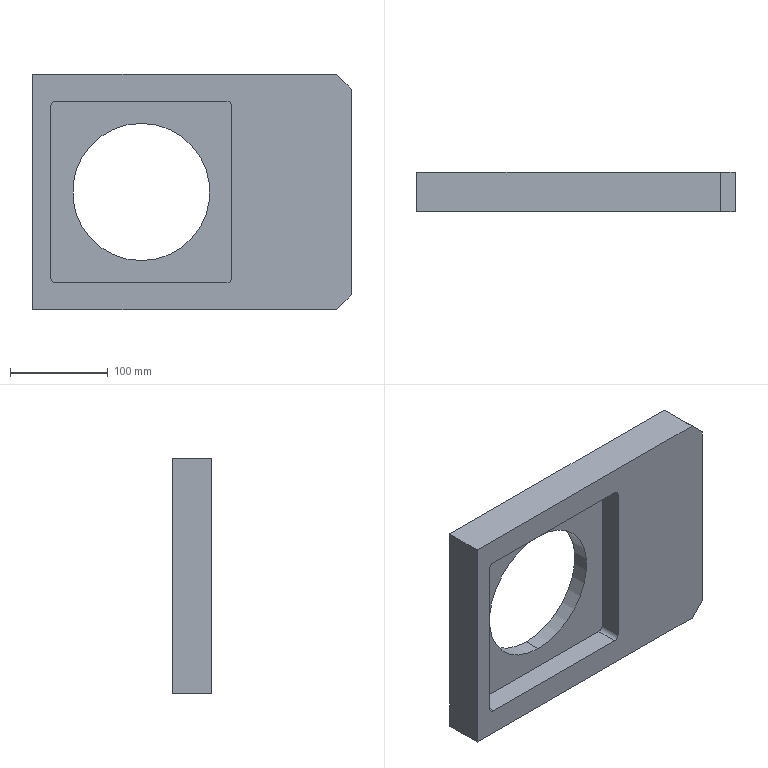Part | SolidWorks | features Cut 2, Chamfer 1, Extrusion 1, Fillet 1 | 1 solid | 19 faces | box 325 x 40 x 240 mm | volume 2062624 mm3 | plane 13 | cylinder 6 | commonest cylinder face diameters 10 x4 140 x2
STEP:
#1=CARTESIAN_POINT('',(-51.794,40.,70.));
#2=VERTEX_POINT('',#1);
#3=CARTESIAN_POINT('',(-51.794,40.,-70.));
#4=VERTEX_POINT('',#3);
#5=CARTESIAN_POINT('',(-51.794,40.,0.));
#6=DIRECTION('',(0.,-1.,0.));
#7=DIRECTION('',(0.,0.,-1.));
#8=AXIS2_PLACEMENT_3D('',#5,#6,#7);
#9=CIRCLE('',#8,70.);
#10=EDGE_CURVE('',#2,#4,#9,.T.);
#11=ORIENTED_EDGE('',*,*,#10,.F.);
#12=CARTESIAN_POINT('',(-51.794,23.,70.));
#13=VERTEX_POINT('',#12);
#14=CARTESIAN_POINT('',(-51.794,40.,70.));
#15=DIRECTION('',(0.,-1.,0.));
#16=VECTOR('',#15,1000.);
#17=LINE('',#14,#16);
#18=EDGE_CURVE('',#2,#13,#17,.T.);
#19=ORIENTED_EDGE('',*,*,#18,.T.);
#20=CARTESIAN_POINT('',(-51.794,23.,-70.));
#21=VERTEX_POINT('',#20);
#22=CARTESIAN_POINT('',(-51.794,23.,0.));
#23=DIRECTION('',(0.,-1.,0.));
#24=DIRECTION('',(0.,0.,-1.));
#25=AXIS2_PLACEMENT_3D('',#22,#23,#24);
#26=CIRCLE('',#25,70.);
#27=EDGE_CURVE('',#13,#21,#26,.T.);
#28=ORIENTED_EDGE('',*,*,#27,.T.);
#29=CARTESIAN_POINT('',(-51.794,40.,-70.));
#30=DIRECTION('',(0.,-1.,0.));
#31=VECTOR('',#30,1000.);
#32=LINE('',#29,#31);
#33=EDGE_CURVE('',#4,#21,#32,.T.);
#34=ORIENTED_EDGE('',*,*,#33,.F.);
#35=EDGE_LOOP('',(#11,#19,#28,#34));
#36=FACE_OUTER_BOUND('',#35,.T.);
#37=CARTESIAN_POINT('',(-51.794,40.,0.));
#38=DIRECTION('',(0.,-1.,0.));
#39=DIRECTION('',(0.,0.,-1.));
#40=AXIS2_PLACEMENT_3D('',#37,#38,#39);
#41=CYLINDRICAL_SURFACE('',#40,70.);
#42=ADVANCED_FACE('',(#36),#41,.F.);
#43=CARTESIAN_POINT('',(162.5,0.,105.));
#44=VERTEX_POINT('',#43);
#45=CARTESIAN_POINT('',(162.5,0.,-105.));
#46=VERTEX_POINT('',#45);
#47=CARTESIAN_POINT('',(162.5,0.,120.));
#48=DIRECTION('',(0.,0.,-1.));
#49=VECTOR('',#48,1000.);
#50=LINE('',#47,#49);
#51=EDGE_CURVE('',#44,#46,#50,.T.);
#52=ORIENTED_EDGE('',*,*,#51,.T.);
#53=CARTESIAN_POINT('',(162.5,40.,-105.));
#54=VERTEX_POINT('',#53);
#55=CARTESIAN_POINT('',(162.5,40.,-105.));
#56=DIRECTION('',(0.,1.,0.));
#57=VECTOR('',#56,1000.);
#58=LINE('',#55,#57);
#59=EDGE_CURVE('',#46,#54,#58,.T.);
#60=ORIENTED_EDGE('',*,*,#59,.T.);
#61=CARTESIAN_POINT('',(162.5,40.,105.));
#62=VERTEX_POINT('',#61);
#63=CARTESIAN_POINT('',(162.5,40.,120.));
#64=DIRECTION('',(0.,0.,-1.));
#65=VECTOR('',#64,1000.);
#66=LINE('',#63,#65);
#67=EDGE_CURVE('',#62,#54,#66,.T.);
#68=ORIENTED_EDGE('',*,*,#67,.F.);
#69=CARTESIAN_POINT('',(162.5,40.,105.));
#70=DIRECTION('',(0.,-1.,0.));
#71=VECTOR('',#70,1000.);
#72=LINE('',#69,#71);
#73=EDGE_CURVE('',#62,#44,#72,.T.);
#74=ORIENTED_EDGE('',*,*,#73,.T.);
#75=EDGE_LOOP('',(#52,#60,#68,#74));
#76=FACE_OUTER_BOUND('',#75,.T.);
#77=CARTESIAN_POINT('',(162.5,40.,120.));
#78=DIRECTION('',(-1.,0.,0.));
#79=DIRECTION('',(0.,0.,1.));
#80=AXIS2_PLACEMENT_3D('',#77,#78,#79);
#81=PLANE('',#80);
#82=ADVANCED_FACE('',(#76),#81,.F.);
#83=CARTESIAN_POINT('',(147.5,40.,-120.));
#84=VERTEX_POINT('',#83);
#85=CARTESIAN_POINT('',(-162.5,40.,-120.));
#86=VERTEX_POINT('',#85);
#87=CARTESIAN_POINT('',(-162.5,40.,-120.));
#88=DIRECTION('',(-1.,0.,0.));
#89=VECTOR('',#88,1000.);
#90=LINE('',#87,#89);
#91=EDGE_CURVE('',#84,#86,#90,.T.);
#92=ORIENTED_EDGE('',*,*,#91,.F.);
#93=CARTESIAN_POINT('',(147.5,0.,-120.));
#94=VERTEX_POINT('',#93);
#95=CARTESIAN_POINT('',(147.5,40.,-120.));
#96=DIRECTION('',(0.,-1.,0.));
#97=VECTOR('',#96,1000.);
#98=LINE('',#95,#97);
#99=EDGE_CURVE('',#84,#94,#98,.T.);
#100=ORIENTED_EDGE('',*,*,#99,.T.);
#101=CARTESIAN_POINT('',(-162.5,0.,-120.));
#102=VERTEX_POINT('',#101);
#103=CARTESIAN_POINT('',(-162.5,0.,-120.));
#104=DIRECTION('',(-1.,0.,0.));
#105=VECTOR('',#104,1000.);
#106=LINE('',#103,#105);
#107=EDGE_CURVE('',#94,#102,#106,.T.);
#108=ORIENTED_EDGE('',*,*,#107,.T.);
#109=CARTESIAN_POINT('',(-162.5,40.,-120.));
#110=DIRECTION('',(0.,-1.,0.));
#111=VECTOR('',#110,1000.);
#112=LINE('',#109,#111);
#113=EDGE_CURVE('',#86,#102,#112,.T.);
#114=ORIENTED_EDGE('',*,*,#113,.F.);
#115=EDGE_LOOP('',(#92,#100,#108,#114));
#116=FACE_OUTER_BOUND('',#115,.T.);
#117=CARTESIAN_POINT('',(-162.5,40.,-120.));
#118=DIRECTION('',(0.,0.,1.));
#119=DIRECTION('',(1.,0.,0.));
#120=AXIS2_PLACEMENT_3D('',#117,#118,#119);
#121=PLANE('',#120);
#122=ADVANCED_FACE('',(#116),#121,.F.);
#123=CARTESIAN_POINT('',(-162.5,0.,120.));
#124=VERTEX_POINT('',#123);
#125=CARTESIAN_POINT('',(-162.5,0.,120.));
#126=DIRECTION('',(0.,0.,1.));
#127=VECTOR('',#126,1000.);
#128=LINE('',#125,#127);
#129=EDGE_CURVE('',#102,#124,#128,.T.);
#130=ORIENTED_EDGE('',*,*,#129,.T.);
#131=CARTESIAN_POINT('',(-162.5,40.,120.));
#132=VERTEX_POINT('',#131);
#133=CARTESIAN_POINT('',(-162.5,40.,120.));
#134=DIRECTION('',(0.,-1.,0.));
#135=VECTOR('',#134,1000.);
#136=LINE('',#133,#135);
#137=EDGE_CURVE('',#132,#124,#136,.T.);
#138=ORIENTED_EDGE('',*,*,#137,.F.);
#139=CARTESIAN_POINT('',(-162.5,40.,120.));
#140=DIRECTION('',(0.,0.,1.));
#141=VECTOR('',#140,1000.);
#142=LINE('',#139,#141);
#143=EDGE_CURVE('',#86,#132,#142,.T.);
#144=ORIENTED_EDGE('',*,*,#143,.F.);
#145=ORIENTED_EDGE('',*,*,#113,.T.);
#146=EDGE_LOOP('',(#130,#138,#144,#145));
#147=FACE_OUTER_BOUND('',#146,.T.);
#148=CARTESIAN_POINT('',(-162.5,40.,120.));
#149=DIRECTION('',(1.,0.,0.));
#150=DIRECTION('',(0.,0.,-1.));
#151=AXIS2_PLACEMENT_3D('',#148,#149,#150);
#152=PLANE('',#151);
#153=ADVANCED_FACE('',(#147),#152,.F.);
#154=CARTESIAN_POINT('',(147.5,0.,120.));
#155=VERTEX_POINT('',#154);
#156=CARTESIAN_POINT('',(-162.5,0.,120.));
#157=DIRECTION('',(1.,0.,0.));
#158=VECTOR('',#157,1000.);
#159=LINE('',#156,#158);
#160=EDGE_CURVE('',#124,#155,#159,.T.);
#161=ORIENTED_EDGE('',*,*,#160,.T.);
#162=CARTESIAN_POINT('',(147.5,40.,120.));
#163=VERTEX_POINT('',#162);
#164=CARTESIAN_POINT('',(147.5,40.,120.));
#165=DIRECTION('',(0.,1.,0.));
#166=VECTOR('',#165,1000.);
#167=LINE('',#164,#166);
#168=EDGE_CURVE('',#155,#163,#167,.T.);
#169=ORIENTED_EDGE('',*,*,#168,.T.);
#170=CARTESIAN_POINT('',(-162.5,40.,120.));
#171=DIRECTION('',(1.,0.,0.));
#172=VECTOR('',#171,1000.);
#173=LINE('',#170,#172);
#174=EDGE_CURVE('',#132,#163,#173,.T.);
#175=ORIENTED_EDGE('',*,*,#174,.F.);
#176=ORIENTED_EDGE('',*,*,#137,.T.);
#177=EDGE_LOOP('',(#161,#169,#175,#176));
#178=FACE_OUTER_BOUND('',#177,.T.);
#179=CARTESIAN_POINT('',(-162.5,40.,120.));
#180=DIRECTION('',(0.,0.,-1.));
#181=DIRECTION('',(-1.,0.,0.));
#182=AXIS2_PLACEMENT_3D('',#179,#180,#181);
#183=PLANE('',#182);
#184=ADVANCED_FACE('',(#178),#183,.F.);
#185=CARTESIAN_POINT('',(-51.794,40.,0.));
#186=DIRECTION('',(0.,-1.,0.));
#187=DIRECTION('',(0.,0.,-1.));
#188=AXIS2_PLACEMENT_3D('',#185,#186,#187);
#189=CIRCLE('',#188,70.);
#190=EDGE_CURVE('',#4,#2,#189,.T.);
#191=ORIENTED_EDGE('',*,*,#190,.T.);
#192=ORIENTED_EDGE('',*,*,#10,.T.);
#193=EDGE_LOOP('',(#191,#192));
#194=FACE_BOUND('',#193,.T.);
#195=ORIENTED_EDGE('',*,*,#67,.T.);
#196=CARTESIAN_POINT('',(147.5,40.,-120.));
#197=DIRECTION('',(-0.7071,0.,-0.7071));
#198=VECTOR('',#197,1000.);
#199=LINE('',#196,#198);
#200=EDGE_CURVE('',#54,#84,#199,.T.);
#201=ORIENTED_EDGE('',*,*,#200,.T.);
#202=ORIENTED_EDGE('',*,*,#91,.T.);
#203=ORIENTED_EDGE('',*,*,#143,.T.);
#204=ORIENTED_EDGE('',*,*,#174,.T.);
#205=CARTESIAN_POINT('',(162.5,40.,105.));
#206=DIRECTION('',(0.7071,0.,-0.7071));
#207=VECTOR('',#206,1000.);
#208=LINE('',#205,#207);
#209=EDGE_CURVE('',#163,#62,#208,.T.);
#210=ORIENTED_EDGE('',*,*,#209,.T.);
#211=EDGE_LOOP('',(#195,#201,#202,#203,#204,#210));
#212=FACE_OUTER_BOUND('',#211,.T.);
#213=CARTESIAN_POINT('',(0.,40.,0.));
#214=DIRECTION('',(0.,-1.,0.));
#215=DIRECTION('',(0.,0.,-1.));
#216=AXIS2_PLACEMENT_3D('',#213,#214,#215);
#217=PLANE('',#216);
#218=ADVANCED_FACE('',(#194,#212),#217,.F.);
#219=CARTESIAN_POINT('',(-144.294,0.,87.5));
#220=VERTEX_POINT('',#219);
#221=CARTESIAN_POINT('',(-144.294,0.,-87.5));
#222=VERTEX_POINT('',#221);
#223=CARTESIAN_POINT('',(-144.294,0.,-92.5));
#224=DIRECTION('',(0.,0.,-1.));
#225=VECTOR('',#224,1000.);
#226=LINE('',#223,#225);
#227=EDGE_CURVE('',#220,#222,#226,.T.);
#228=ORIENTED_EDGE('',*,*,#227,.F.);
#229=CARTESIAN_POINT('',(-139.294,0.,92.5));
#230=VERTEX_POINT('',#229);
#231=CARTESIAN_POINT('',(-139.294,0.,87.5));
#232=DIRECTION('',(0.,1.,0.));
#233=DIRECTION('',(0.,0.,-1.));
#234=AXIS2_PLACEMENT_3D('',#231,#232,#233);
#235=CIRCLE('',#234,5.);
#236=EDGE_CURVE('',#220,#230,#235,.T.);
#237=ORIENTED_EDGE('',*,*,#236,.T.);
#238=CARTESIAN_POINT('',(35.706,0.,92.5));
#239=VERTEX_POINT('',#238);
#240=CARTESIAN_POINT('',(40.706,0.,92.5));
#241=DIRECTION('',(-1.,0.,0.));
#242=VECTOR('',#241,1000.);
#243=LINE('',#240,#242);
#244=EDGE_CURVE('',#239,#230,#243,.T.);
#245=ORIENTED_EDGE('',*,*,#244,.F.);
#246=CARTESIAN_POINT('',(40.706,0.,87.5));
#247=VERTEX_POINT('',#246);
#248=CARTESIAN_POINT('',(35.706,0.,87.5));
#249=DIRECTION('',(0.,1.,0.));
#250=DIRECTION('',(0.,0.,-1.));
#251=AXIS2_PLACEMENT_3D('',#248,#249,#250);
#252=CIRCLE('',#251,5.);
#253=EDGE_CURVE('',#239,#247,#252,.T.);
#254=ORIENTED_EDGE('',*,*,#253,.T.);
#255=CARTESIAN_POINT('',(40.706,0.,-87.5));
#256=VERTEX_POINT('',#255);
#257=CARTESIAN_POINT('',(40.706,0.,-92.5));
#258=DIRECTION('',(0.,0.,1.));
#259=VECTOR('',#258,1000.);
#260=LINE('',#257,#259);
#261=EDGE_CURVE('',#256,#247,#260,.T.);
#262=ORIENTED_EDGE('',*,*,#261,.F.);
#263=CARTESIAN_POINT('',(35.706,0.,-92.5));
#264=VERTEX_POINT('',#263);
#265=CARTESIAN_POINT('',(35.706,0.,-87.5));
#266=DIRECTION('',(0.,1.,0.));
#267=DIRECTION('',(0.,0.,-1.));
#268=AXIS2_PLACEMENT_3D('',#265,#266,#267);
#269=CIRCLE('',#268,5.);
#270=EDGE_CURVE('',#256,#264,#269,.T.);
#271=ORIENTED_EDGE('',*,*,#270,.T.);
#272=CARTESIAN_POINT('',(-139.294,0.,-92.5));
#273=VERTEX_POINT('',#272);
#274=CARTESIAN_POINT('',(40.706,0.,-92.5));
#275=DIRECTION('',(1.,0.,0.));
#276=VECTOR('',#275,1000.);
#277=LINE('',#274,#276);
#278=EDGE_CURVE('',#273,#264,#277,.T.);
#279=ORIENTED_EDGE('',*,*,#278,.F.);
#280=CARTESIAN_POINT('',(-139.294,0.,-87.5));
#281=DIRECTION('',(0.,1.,0.));
#282=DIRECTION('',(0.,0.,-1.));
#283=AXIS2_PLACEMENT_3D('',#280,#281,#282);
#284=CIRCLE('',#283,5.);
#285=EDGE_CURVE('',#273,#222,#284,.T.);
#286=ORIENTED_EDGE('',*,*,#285,.T.);
#287=EDGE_LOOP('',(#228,#237,#245,#254,#262,#271,#279,#286));
#288=FACE_BOUND('',#287,.T.);
#289=ORIENTED_EDGE('',*,*,#107,.F.);
#290=CARTESIAN_POINT('',(133.75,0.,-133.75));
#291=DIRECTION('',(0.7071,0.,0.7071));
#292=VECTOR('',#291,1000.);
#293=LINE('',#290,#292);
#294=EDGE_CURVE('',#94,#46,#293,.T.);
#295=ORIENTED_EDGE('',*,*,#294,.T.);
#296=ORIENTED_EDGE('',*,*,#51,.F.);
#297=CARTESIAN_POINT('',(133.75,0.,133.75));
#298=DIRECTION('',(-0.7071,0.,0.7071));
#299=VECTOR('',#298,1000.);
#300=LINE('',#297,#299);
#301=EDGE_CURVE('',#44,#155,#300,.T.);
#302=ORIENTED_EDGE('',*,*,#301,.T.);
#303=ORIENTED_EDGE('',*,*,#160,.F.);
#304=ORIENTED_EDGE('',*,*,#129,.F.);
#305=EDGE_LOOP('',(#289,#295,#296,#302,#303,#304));
#306=FACE_OUTER_BOUND('',#305,.T.);
#307=CARTESIAN_POINT('',(0.,0.,0.));
#308=DIRECTION('',(0.,-1.,0.));
#309=DIRECTION('',(0.,0.,-1.));
#310=AXIS2_PLACEMENT_3D('',#307,#308,#309);
#311=PLANE('',#310);
#312=ADVANCED_FACE('',(#288,#306),#311,.T.);
#313=CARTESIAN_POINT('',(-144.294,23.,87.5));
#314=VERTEX_POINT('',#313);
#315=CARTESIAN_POINT('',(-144.294,23.,-87.5));
#316=VERTEX_POINT('',#315);
#317=CARTESIAN_POINT('',(-144.294,23.,-92.5));
#318=DIRECTION('',(0.,0.,-1.));
#319=VECTOR('',#318,1000.);
#320=LINE('',#317,#319);
#321=EDGE_CURVE('',#314,#316,#320,.T.);
#322=ORIENTED_EDGE('',*,*,#321,.F.);
#323=CARTESIAN_POINT('',(-144.294,0.,87.5));
#324=DIRECTION('',(0.,-1.,0.));
#325=VECTOR('',#324,1000.);
#326=LINE('',#323,#325);
#327=EDGE_CURVE('',#314,#220,#326,.T.);
#328=ORIENTED_EDGE('',*,*,#327,.T.);
#329=ORIENTED_EDGE('',*,*,#227,.T.);
#330=CARTESIAN_POINT('',(-144.294,23.,-87.5));
#331=DIRECTION('',(0.,1.,0.));
#332=VECTOR('',#331,1000.);
#333=LINE('',#330,#332);
#334=EDGE_CURVE('',#222,#316,#333,.T.);
#335=ORIENTED_EDGE('',*,*,#334,.T.);
#336=EDGE_LOOP('',(#322,#328,#329,#335));
#337=FACE_OUTER_BOUND('',#336,.T.);
#338=CARTESIAN_POINT('',(-144.294,23.,-92.5));
#339=DIRECTION('',(-1.,0.,0.));
#340=DIRECTION('',(0.,0.,1.));
#341=AXIS2_PLACEMENT_3D('',#338,#339,#340);
#342=PLANE('',#341);
#343=ADVANCED_FACE('',(#337),#342,.F.);
#344=ORIENTED_EDGE('',*,*,#244,.T.);
#345=CARTESIAN_POINT('',(-139.294,23.,92.5));
#346=VERTEX_POINT('',#345);
#347=CARTESIAN_POINT('',(-139.294,23.,92.5));
#348=DIRECTION('',(0.,1.,0.));
#349=VECTOR('',#348,1000.);
#350=LINE('',#347,#349);
#351=EDGE_CURVE('',#230,#346,#350,.T.);
#352=ORIENTED_EDGE('',*,*,#351,.T.);
#353=CARTESIAN_POINT('',(35.706,23.,92.5));
#354=VERTEX_POINT('',#353);
#355=CARTESIAN_POINT('',(40.706,23.,92.5));
#356=DIRECTION('',(-1.,0.,0.));
#357=VECTOR('',#356,1000.);
#358=LINE('',#355,#357);
#359=EDGE_CURVE('',#354,#346,#358,.T.);
#360=ORIENTED_EDGE('',*,*,#359,.F.);
#361=CARTESIAN_POINT('',(35.706,0.,92.5));
#362=DIRECTION('',(0.,-1.,0.));
#363=VECTOR('',#362,1000.);
#364=LINE('',#361,#363);
#365=EDGE_CURVE('',#354,#239,#364,.T.);
#366=ORIENTED_EDGE('',*,*,#365,.T.);
#367=EDGE_LOOP('',(#344,#352,#360,#366));
#368=FACE_OUTER_BOUND('',#367,.T.);
#369=CARTESIAN_POINT('',(40.706,23.,92.5));
#370=DIRECTION('',(0.,0.,1.));
#371=DIRECTION('',(1.,0.,0.));
#372=AXIS2_PLACEMENT_3D('',#369,#370,#371);
#373=PLANE('',#372);
#374=ADVANCED_FACE('',(#368),#373,.F.);
#375=ORIENTED_EDGE('',*,*,#261,.T.);
#376=CARTESIAN_POINT('',(40.706,23.,87.5));
#377=VERTEX_POINT('',#376);
#378=CARTESIAN_POINT('',(40.706,23.,87.5));
#379=DIRECTION('',(0.,1.,0.));
#380=VECTOR('',#379,1000.);
#381=LINE('',#378,#380);
#382=EDGE_CURVE('',#247,#377,#381,.T.);
#383=ORIENTED_EDGE('',*,*,#382,.T.);
#384=CARTESIAN_POINT('',(40.706,23.,-87.5));
#385=VERTEX_POINT('',#384);
#386=CARTESIAN_POINT('',(40.706,23.,-92.5));
#387=DIRECTION('',(0.,0.,1.));
#388=VECTOR('',#387,1000.);
#389=LINE('',#386,#388);
#390=EDGE_CURVE('',#385,#377,#389,.T.);
#391=ORIENTED_EDGE('',*,*,#390,.F.);
#392=CARTESIAN_POINT('',(40.706,0.,-87.5));
#393=DIRECTION('',(0.,-1.,0.));
#394=VECTOR('',#393,1000.);
#395=LINE('',#392,#394);
#396=EDGE_CURVE('',#385,#256,#395,.T.);
#397=ORIENTED_EDGE('',*,*,#396,.T.);
#398=EDGE_LOOP('',(#375,#383,#391,#397));
#399=FACE_OUTER_BOUND('',#398,.T.);
#400=CARTESIAN_POINT('',(40.706,23.,-92.5));
#401=DIRECTION('',(1.,0.,0.));
#402=DIRECTION('',(0.,0.,-1.));
#403=AXIS2_PLACEMENT_3D('',#400,#401,#402);
#404=PLANE('',#403);
#405=ADVANCED_FACE('',(#399),#404,.F.);
#406=ORIENTED_EDGE('',*,*,#278,.T.);
#407=CARTESIAN_POINT('',(35.706,23.,-92.5));
#408=VERTEX_POINT('',#407);
#409=CARTESIAN_POINT('',(35.706,23.,-92.5));
#410=DIRECTION('',(0.,1.,0.));
#411=VECTOR('',#410,1000.);
#412=LINE('',#409,#411);
#413=EDGE_CURVE('',#264,#408,#412,.T.);
#414=ORIENTED_EDGE('',*,*,#413,.T.);
#415=CARTESIAN_POINT('',(-139.294,23.,-92.5));
#416=VERTEX_POINT('',#415);
#417=CARTESIAN_POINT('',(40.706,23.,-92.5));
#418=DIRECTION('',(1.,0.,0.));
#419=VECTOR('',#418,1000.);
#420=LINE('',#417,#419);
#421=EDGE_CURVE('',#416,#408,#420,.T.);
#422=ORIENTED_EDGE('',*,*,#421,.F.);
#423=CARTESIAN_POINT('',(-139.294,0.,-92.5));
#424=DIRECTION('',(0.,-1.,0.));
#425=VECTOR('',#424,1000.);
#426=LINE('',#423,#425);
#427=EDGE_CURVE('',#416,#273,#426,.T.);
#428=ORIENTED_EDGE('',*,*,#427,.T.);
#429=EDGE_LOOP('',(#406,#414,#422,#428));
#430=FACE_OUTER_BOUND('',#429,.T.);
#431=CARTESIAN_POINT('',(40.706,23.,-92.5));
#432=DIRECTION('',(0.,0.,-1.));
#433=DIRECTION('',(-1.,0.,0.));
#434=AXIS2_PLACEMENT_3D('',#431,#432,#433);
#435=PLANE('',#434);
#436=ADVANCED_FACE('',(#430),#435,.F.);
#437=CARTESIAN_POINT('',(-51.794,23.,0.));
#438=DIRECTION('',(0.,-1.,0.));
#439=DIRECTION('',(0.,0.,-1.));
#440=AXIS2_PLACEMENT_3D('',#437,#438,#439);
#441=CIRCLE('',#440,70.);
#442=EDGE_CURVE('',#21,#13,#441,.T.);
#443=ORIENTED_EDGE('',*,*,#442,.F.);
#444=ORIENTED_EDGE('',*,*,#27,.F.);
#445=EDGE_LOOP('',(#443,#444));
#446=FACE_BOUND('',#445,.T.);
#447=ORIENTED_EDGE('',*,*,#359,.T.);
#448=CARTESIAN_POINT('',(-139.294,23.,87.5));
#449=DIRECTION('',(0.,-1.,0.));
#450=DIRECTION('',(0.,0.,-1.));
#451=AXIS2_PLACEMENT_3D('',#448,#449,#450);
#452=CIRCLE('',#451,5.);
#453=EDGE_CURVE('',#346,#314,#452,.T.);
#454=ORIENTED_EDGE('',*,*,#453,.T.);
#455=ORIENTED_EDGE('',*,*,#321,.T.);
#456=CARTESIAN_POINT('',(-139.294,23.,-87.5));
#457=DIRECTION('',(0.,-1.,0.));
#458=DIRECTION('',(0.,0.,-1.));
#459=AXIS2_PLACEMENT_3D('',#456,#457,#458);
#460=CIRCLE('',#459,5.);
#461=EDGE_CURVE('',#316,#416,#460,.T.);
#462=ORIENTED_EDGE('',*,*,#461,.T.);
#463=ORIENTED_EDGE('',*,*,#421,.T.);
#464=CARTESIAN_POINT('',(35.706,23.,-87.5));
#465=DIRECTION('',(0.,-1.,0.));
#466=DIRECTION('',(0.,0.,-1.));
#467=AXIS2_PLACEMENT_3D('',#464,#465,#466);
#468=CIRCLE('',#467,5.);
#469=EDGE_CURVE('',#408,#385,#468,.T.);
#470=ORIENTED_EDGE('',*,*,#469,.T.);
#471=ORIENTED_EDGE('',*,*,#390,.T.);
#472=CARTESIAN_POINT('',(35.706,23.,87.5));
#473=DIRECTION('',(0.,-1.,0.));
#474=DIRECTION('',(0.,0.,-1.));
#475=AXIS2_PLACEMENT_3D('',#472,#473,#474);
#476=CIRCLE('',#475,5.);
#477=EDGE_CURVE('',#377,#354,#476,.T.);
#478=ORIENTED_EDGE('',*,*,#477,.T.);
#479=EDGE_LOOP('',(#447,#454,#455,#462,#463,#470,#471,#478));
#480=FACE_OUTER_BOUND('',#479,.T.);
#481=CARTESIAN_POINT('',(0.,23.,0.));
#482=DIRECTION('',(0.,-1.,0.));
#483=DIRECTION('',(0.,0.,-1.));
#484=AXIS2_PLACEMENT_3D('',#481,#482,#483);
#485=PLANE('',#484);
#486=ADVANCED_FACE('',(#446,#480),#485,.T.);
#487=ORIENTED_EDGE('',*,*,#18,.F.);
#488=ORIENTED_EDGE('',*,*,#190,.F.);
#489=ORIENTED_EDGE('',*,*,#33,.T.);
#490=ORIENTED_EDGE('',*,*,#442,.T.);
#491=EDGE_LOOP('',(#487,#488,#489,#490));
#492=FACE_OUTER_BOUND('',#491,.T.);
#493=CARTESIAN_POINT('',(-51.794,40.,0.));
#494=DIRECTION('',(0.,-1.,0.));
#495=DIRECTION('',(0.,0.,-1.));
#496=AXIS2_PLACEMENT_3D('',#493,#494,#495);
#497=CYLINDRICAL_SURFACE('',#496,70.);
#498=ADVANCED_FACE('',(#492),#497,.F.);
#499=ORIENTED_EDGE('',*,*,#453,.F.);
#500=ORIENTED_EDGE('',*,*,#351,.F.);
#501=ORIENTED_EDGE('',*,*,#236,.F.);
#502=ORIENTED_EDGE('',*,*,#327,.F.);
#503=EDGE_LOOP('',(#499,#500,#501,#502));
#504=FACE_OUTER_BOUND('',#503,.T.);
#505=CARTESIAN_POINT('',(-139.294,23.,87.5));
#506=DIRECTION('',(0.,1.,0.));
#507=DIRECTION('',(0.,0.,1.));
#508=AXIS2_PLACEMENT_3D('',#505,#506,#507);
#509=CYLINDRICAL_SURFACE('',#508,5.);
#510=ADVANCED_FACE('',(#504),#509,.F.);
#511=ORIENTED_EDGE('',*,*,#477,.F.);
#512=ORIENTED_EDGE('',*,*,#382,.F.);
#513=ORIENTED_EDGE('',*,*,#253,.F.);
#514=ORIENTED_EDGE('',*,*,#365,.F.);
#515=EDGE_LOOP('',(#511,#512,#513,#514));
#516=FACE_OUTER_BOUND('',#515,.T.);
#517=CARTESIAN_POINT('',(35.706,23.,87.5));
#518=DIRECTION('',(0.,1.,0.));
#519=DIRECTION('',(0.,0.,1.));
#520=AXIS2_PLACEMENT_3D('',#517,#518,#519);
#521=CYLINDRICAL_SURFACE('',#520,5.);
#522=ADVANCED_FACE('',(#516),#521,.F.);
#523=ORIENTED_EDGE('',*,*,#469,.F.);
#524=ORIENTED_EDGE('',*,*,#413,.F.);
#525=ORIENTED_EDGE('',*,*,#270,.F.);
#526=ORIENTED_EDGE('',*,*,#396,.F.);
#527=EDGE_LOOP('',(#523,#524,#525,#526));
#528=FACE_OUTER_BOUND('',#527,.T.);
#529=CARTESIAN_POINT('',(35.706,23.,-87.5));
#530=DIRECTION('',(0.,1.,0.));
#531=DIRECTION('',(0.,0.,1.));
#532=AXIS2_PLACEMENT_3D('',#529,#530,#531);
#533=CYLINDRICAL_SURFACE('',#532,5.);
#534=ADVANCED_FACE('',(#528),#533,.F.);
#535=ORIENTED_EDGE('',*,*,#461,.F.);
#536=ORIENTED_EDGE('',*,*,#334,.F.);
#537=ORIENTED_EDGE('',*,*,#285,.F.);
#538=ORIENTED_EDGE('',*,*,#427,.F.);
#539=EDGE_LOOP('',(#535,#536,#537,#538));
#540=FACE_OUTER_BOUND('',#539,.T.);
#541=CARTESIAN_POINT('',(-139.294,23.,-87.5));
#542=DIRECTION('',(0.,1.,0.));
#543=DIRECTION('',(0.,0.,1.));
#544=AXIS2_PLACEMENT_3D('',#541,#542,#543);
#545=CYLINDRICAL_SURFACE('',#544,5.);
#546=ADVANCED_FACE('',(#540),#545,.F.);
#547=ORIENTED_EDGE('',*,*,#200,.F.);
#548=ORIENTED_EDGE('',*,*,#59,.F.);
#549=ORIENTED_EDGE('',*,*,#294,.F.);
#550=ORIENTED_EDGE('',*,*,#99,.F.);
#551=EDGE_LOOP('',(#547,#548,#549,#550));
#552=FACE_OUTER_BOUND('',#551,.T.);
#553=CARTESIAN_POINT('',(147.5,40.,-120.));
#554=DIRECTION('',(-0.7071,0.,0.7071));
#555=DIRECTION('',(0.,-1.,0.));
#556=AXIS2_PLACEMENT_3D('',#553,#554,#555);
#557=PLANE('',#556);
#558=ADVANCED_FACE('',(#552),#557,.F.);
#559=ORIENTED_EDGE('',*,*,#209,.F.);
#560=ORIENTED_EDGE('',*,*,#168,.F.);
#561=ORIENTED_EDGE('',*,*,#301,.F.);
#562=ORIENTED_EDGE('',*,*,#73,.F.);
#563=EDGE_LOOP('',(#559,#560,#561,#562));
#564=FACE_OUTER_BOUND('',#563,.T.);
#565=CARTESIAN_POINT('',(162.5,40.,105.));
#566=DIRECTION('',(-0.7071,0.,-0.7071));
#567=DIRECTION('',(0.,-1.,0.));
#568=AXIS2_PLACEMENT_3D('',#565,#566,#567);
#569=PLANE('',#568);
#570=ADVANCED_FACE('',(#564),#569,.F.);
#571=CLOSED_SHELL('',(#42,#82,#122,#153,#184,#218,#312,#343,#374,#405,#436,#486,#498,#510,#522,#534,#546,#558,#570));
#572=MANIFOLD_SOLID_BREP('',#571);
#573=CARTESIAN_POINT('',(0.,0.,0.));
#574=DIRECTION('',(0.,0.,1.));
#575=DIRECTION('',(1.,0.,0.));
#576=AXIS2_PLACEMENT_3D('',#573,#574,#575);
#577=(LENGTH_UNIT()NAMED_UNIT(*)SI_UNIT(.MILLI.,.METRE.));
#578=UNCERTAINTY_MEASURE_WITH_UNIT(LENGTH_MEASURE(0.00001),#577,'','');
#579=(NAMED_UNIT(*)PLANE_ANGLE_UNIT()SI_UNIT($,.RADIAN.));
#580=(NAMED_UNIT(*)SI_UNIT($,.STERADIAN.)SOLID_ANGLE_UNIT());
#581=(GEOMETRIC_REPRESENTATION_CONTEXT(3)GLOBAL_UNCERTAINTY_ASSIGNED_CONTEXT((#578))GLOBAL_UNIT_ASSIGNED_CONTEXT((#577,#579,#580))REPRESENTATION_CONTEXT('',''));
#582=ADVANCED_BREP_SHAPE_REPRESENTATION('',(#572,#576),#581);